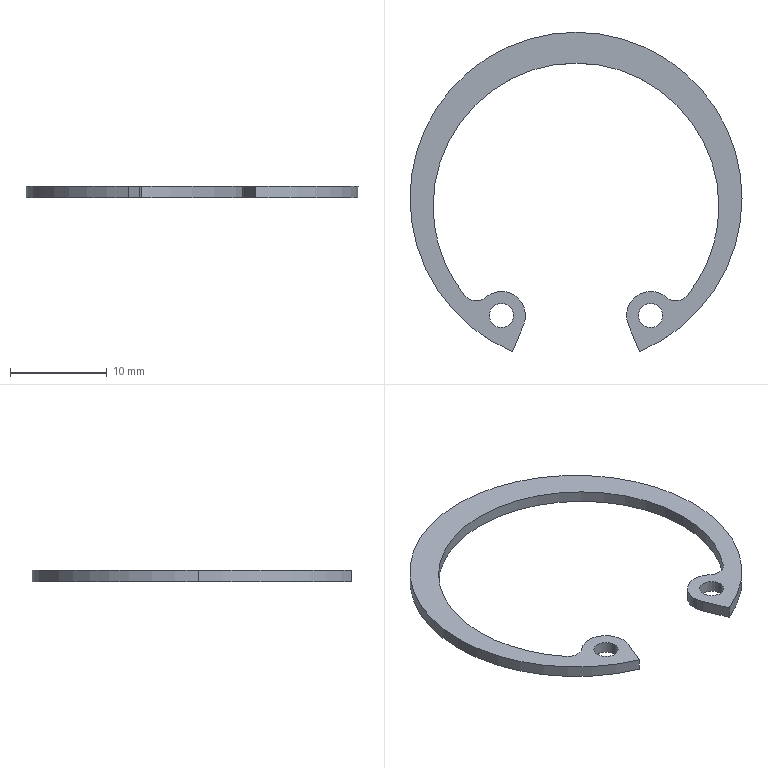Part | SolidWorks | features Extrusion 1 | 1 solid | 19 faces | box 34.4 x 33.091 x 1.2 mm | volume 290.13 mm3 | cylinder 15 | plane 4 | commonest cylinder face diameters 2.5 x4 5 x3 29.6 x3 34.4 x3 3 x2
STEP:
#1=CARTESIAN_POINT('',(6.487,-12.145,-1.2));
#2=VERTEX_POINT('',#1);
#3=CARTESIAN_POINT('',(8.987,-12.145,-1.2));
#4=VERTEX_POINT('',#3);
#5=CARTESIAN_POINT('',(7.737,-12.145,-1.2));
#6=DIRECTION('',(0.,0.,1.));
#7=DIRECTION('',(-1.,0.,0.));
#8=AXIS2_PLACEMENT_3D('',#5,#6,#7);
#9=CIRCLE('',#8,1.25);
#10=EDGE_CURVE('',#2,#4,#9,.T.);
#11=ORIENTED_EDGE('',*,*,#10,.F.);
#12=CARTESIAN_POINT('',(6.487,-12.145,0.));
#13=VERTEX_POINT('',#12);
#14=CARTESIAN_POINT('',(6.487,-12.145,-1.2));
#15=DIRECTION('',(0.,0.,1.));
#16=VECTOR('',#15,1000.);
#17=LINE('',#14,#16);
#18=EDGE_CURVE('',#2,#13,#17,.T.);
#19=ORIENTED_EDGE('',*,*,#18,.T.);
#20=CARTESIAN_POINT('',(8.987,-12.145,0.));
#21=VERTEX_POINT('',#20);
#22=CARTESIAN_POINT('',(7.737,-12.145,0.));
#23=DIRECTION('',(0.,0.,1.));
#24=DIRECTION('',(-1.,0.,0.));
#25=AXIS2_PLACEMENT_3D('',#22,#23,#24);
#26=CIRCLE('',#25,1.25);
#27=EDGE_CURVE('',#13,#21,#26,.T.);
#28=ORIENTED_EDGE('',*,*,#27,.T.);
#29=CARTESIAN_POINT('',(8.987,-12.145,-1.2));
#30=DIRECTION('',(0.,0.,1.));
#31=VECTOR('',#30,1000.);
#32=LINE('',#29,#31);
#33=EDGE_CURVE('',#4,#21,#32,.T.);
#34=ORIENTED_EDGE('',*,*,#33,.F.);
#35=EDGE_LOOP('',(#11,#19,#28,#34));
#36=FACE_OUTER_BOUND('',#35,.T.);
#37=CARTESIAN_POINT('',(7.737,-12.145,-1.2));
#38=DIRECTION('',(0.,0.,1.));
#39=DIRECTION('',(1.,0.,0.));
#40=AXIS2_PLACEMENT_3D('',#37,#38,#39);
#41=CYLINDRICAL_SURFACE('',#40,1.25);
#42=ADVANCED_FACE('',(#36),#41,.F.);
#43=CARTESIAN_POINT('',(-8.987,-12.145,-1.2));
#44=VERTEX_POINT('',#43);
#45=CARTESIAN_POINT('',(-6.487,-12.145,-1.2));
#46=VERTEX_POINT('',#45);
#47=CARTESIAN_POINT('',(-7.737,-12.145,-1.2));
#48=DIRECTION('',(0.,0.,1.));
#49=DIRECTION('',(-1.,0.,0.));
#50=AXIS2_PLACEMENT_3D('',#47,#48,#49);
#51=CIRCLE('',#50,1.25);
#52=EDGE_CURVE('',#44,#46,#51,.T.);
#53=ORIENTED_EDGE('',*,*,#52,.F.);
#54=CARTESIAN_POINT('',(-8.987,-12.145,0.));
#55=VERTEX_POINT('',#54);
#56=CARTESIAN_POINT('',(-8.987,-12.145,-1.2));
#57=DIRECTION('',(0.,0.,1.));
#58=VECTOR('',#57,1000.);
#59=LINE('',#56,#58);
#60=EDGE_CURVE('',#44,#55,#59,.T.);
#61=ORIENTED_EDGE('',*,*,#60,.T.);
#62=CARTESIAN_POINT('',(-6.487,-12.145,0.));
#63=VERTEX_POINT('',#62);
#64=CARTESIAN_POINT('',(-7.737,-12.145,0.));
#65=DIRECTION('',(0.,0.,1.));
#66=DIRECTION('',(-1.,0.,0.));
#67=AXIS2_PLACEMENT_3D('',#64,#65,#66);
#68=CIRCLE('',#67,1.25);
#69=EDGE_CURVE('',#55,#63,#68,.T.);
#70=ORIENTED_EDGE('',*,*,#69,.T.);
#71=CARTESIAN_POINT('',(-6.487,-12.145,-1.2));
#72=DIRECTION('',(0.,0.,1.));
#73=VECTOR('',#72,1000.);
#74=LINE('',#71,#73);
#75=EDGE_CURVE('',#46,#63,#74,.T.);
#76=ORIENTED_EDGE('',*,*,#75,.F.);
#77=EDGE_LOOP('',(#53,#61,#70,#76));
#78=FACE_OUTER_BOUND('',#77,.T.);
#79=CARTESIAN_POINT('',(-7.737,-12.145,-1.2));
#80=DIRECTION('',(0.,0.,1.));
#81=DIRECTION('',(1.,0.,0.));
#82=AXIS2_PLACEMENT_3D('',#79,#80,#81);
#83=CYLINDRICAL_SURFACE('',#82,1.25);
#84=ADVANCED_FACE('',(#78),#83,.F.);
#85=CARTESIAN_POINT('',(17.2,0.,-1.2));
#86=VERTEX_POINT('',#85);
#87=CARTESIAN_POINT('',(-17.2,0.,-1.2));
#88=VERTEX_POINT('',#87);
#89=CARTESIAN_POINT('',(0.,0.,-1.2));
#90=DIRECTION('',(0.,0.,1.));
#91=DIRECTION('',(1.,0.,0.));
#92=AXIS2_PLACEMENT_3D('',#89,#90,#91);
#93=CIRCLE('',#92,17.2);
#94=EDGE_CURVE('',#86,#88,#93,.T.);
#95=ORIENTED_EDGE('',*,*,#94,.T.);
#96=CARTESIAN_POINT('',(-17.2,0.,0.));
#97=VERTEX_POINT('',#96);
#98=CARTESIAN_POINT('',(-17.2,0.,-1.2));
#99=DIRECTION('',(0.,0.,1.));
#100=VECTOR('',#99,1000.);
#101=LINE('',#98,#100);
#102=EDGE_CURVE('',#88,#97,#101,.T.);
#103=ORIENTED_EDGE('',*,*,#102,.T.);
#104=CARTESIAN_POINT('',(17.2,0.,0.));
#105=VERTEX_POINT('',#104);
#106=CARTESIAN_POINT('',(0.,0.,0.));
#107=DIRECTION('',(0.,0.,1.));
#108=DIRECTION('',(1.,0.,0.));
#109=AXIS2_PLACEMENT_3D('',#106,#107,#108);
#110=CIRCLE('',#109,17.2);
#111=EDGE_CURVE('',#105,#97,#110,.T.);
#112=ORIENTED_EDGE('',*,*,#111,.F.);
#113=CARTESIAN_POINT('',(17.2,0.,-1.2));
#114=DIRECTION('',(0.,0.,1.));
#115=VECTOR('',#114,1000.);
#116=LINE('',#113,#115);
#117=EDGE_CURVE('',#86,#105,#116,.T.);
#118=ORIENTED_EDGE('',*,*,#117,.F.);
#119=EDGE_LOOP('',(#95,#103,#112,#118));
#120=FACE_OUTER_BOUND('',#119,.T.);
#121=CARTESIAN_POINT('',(0.,0.,-1.2));
#122=DIRECTION('',(0.,0.,1.));
#123=DIRECTION('',(1.,0.,0.));
#124=AXIS2_PLACEMENT_3D('',#121,#122,#123);
#125=CYLINDRICAL_SURFACE('',#124,17.2);
#126=ADVANCED_FACE('',(#120),#125,.T.);
#127=CARTESIAN_POINT('',(6.582,-15.891,-1.2));
#128=VERTEX_POINT('',#127);
#129=CARTESIAN_POINT('',(0.,0.,-1.2));
#130=DIRECTION('',(0.,0.,1.));
#131=DIRECTION('',(1.,0.,0.));
#132=AXIS2_PLACEMENT_3D('',#129,#130,#131);
#133=CIRCLE('',#132,17.2);
#134=EDGE_CURVE('',#128,#86,#133,.T.);
#135=ORIENTED_EDGE('',*,*,#134,.T.);
#136=ORIENTED_EDGE('',*,*,#117,.T.);
#137=CARTESIAN_POINT('',(6.582,-15.891,0.));
#138=VERTEX_POINT('',#137);
#139=CARTESIAN_POINT('',(0.,0.,0.));
#140=DIRECTION('',(0.,0.,1.));
#141=DIRECTION('',(1.,0.,0.));
#142=AXIS2_PLACEMENT_3D('',#139,#140,#141);
#143=CIRCLE('',#142,17.2);
#144=EDGE_CURVE('',#138,#105,#143,.T.);
#145=ORIENTED_EDGE('',*,*,#144,.F.);
#146=CARTESIAN_POINT('',(6.582,-15.891,-1.2));
#147=DIRECTION('',(0.,0.,1.));
#148=VECTOR('',#147,1000.);
#149=LINE('',#146,#148);
#150=EDGE_CURVE('',#128,#138,#149,.T.);
#151=ORIENTED_EDGE('',*,*,#150,.F.);
#152=EDGE_LOOP('',(#135,#136,#145,#151));
#153=FACE_OUTER_BOUND('',#152,.T.);
#154=CARTESIAN_POINT('',(0.,0.,-1.2));
#155=DIRECTION('',(0.,0.,1.));
#156=DIRECTION('',(1.,0.,0.));
#157=AXIS2_PLACEMENT_3D('',#154,#155,#156);
#158=CYLINDRICAL_SURFACE('',#157,17.2);
#159=ADVANCED_FACE('',(#153),#158,.T.);
#160=CARTESIAN_POINT('',(-5.427,-13.102,-1.2));
#161=VERTEX_POINT('',#160);
#162=CARTESIAN_POINT('',(-5.237,-12.145,-1.2));
#163=VERTEX_POINT('',#162);
#164=CARTESIAN_POINT('',(-7.737,-12.145,-1.2));
#165=DIRECTION('',(0.,0.,1.));
#166=DIRECTION('',(1.,0.,0.));
#167=AXIS2_PLACEMENT_3D('',#164,#165,#166);
#168=CIRCLE('',#167,2.5);
#169=EDGE_CURVE('',#161,#163,#168,.T.);
#170=ORIENTED_EDGE('',*,*,#169,.T.);
#171=CARTESIAN_POINT('',(-5.237,-12.145,0.));
#172=VERTEX_POINT('',#171);
#173=CARTESIAN_POINT('',(-5.237,-12.145,-1.2));
#174=DIRECTION('',(0.,0.,1.));
#175=VECTOR('',#174,1000.);
#176=LINE('',#173,#175);
#177=EDGE_CURVE('',#163,#172,#176,.T.);
#178=ORIENTED_EDGE('',*,*,#177,.T.);
#179=CARTESIAN_POINT('',(-5.427,-13.102,0.));
#180=VERTEX_POINT('',#179);
#181=CARTESIAN_POINT('',(-7.737,-12.145,0.));
#182=DIRECTION('',(0.,0.,1.));
#183=DIRECTION('',(1.,0.,0.));
#184=AXIS2_PLACEMENT_3D('',#181,#182,#183);
#185=CIRCLE('',#184,2.5);
#186=EDGE_CURVE('',#180,#172,#185,.T.);
#187=ORIENTED_EDGE('',*,*,#186,.F.);
#188=CARTESIAN_POINT('',(-5.427,-13.102,-1.2));
#189=DIRECTION('',(0.,0.,1.));
#190=VECTOR('',#189,1000.);
#191=LINE('',#188,#190);
#192=EDGE_CURVE('',#161,#180,#191,.T.);
#193=ORIENTED_EDGE('',*,*,#192,.F.);
#194=EDGE_LOOP('',(#170,#178,#187,#193));
#195=FACE_OUTER_BOUND('',#194,.T.);
#196=CARTESIAN_POINT('',(-7.737,-12.145,-1.2));
#197=DIRECTION('',(0.,0.,1.));
#198=DIRECTION('',(1.,0.,0.));
#199=AXIS2_PLACEMENT_3D('',#196,#197,#198);
#200=CYLINDRICAL_SURFACE('',#199,2.5);
#201=ADVANCED_FACE('',(#195),#200,.T.);
#202=CARTESIAN_POINT('',(-11.536,-10.071,-1.2));
#203=VERTEX_POINT('',#202);
#204=CARTESIAN_POINT('',(-14.8,-0.8,-1.2));
#205=VERTEX_POINT('',#204);
#206=CARTESIAN_POINT('',(0.,-0.8,-1.2));
#207=DIRECTION('',(0.,0.,-1.));
#208=DIRECTION('',(-1.,0.,0.));
#209=AXIS2_PLACEMENT_3D('',#206,#207,#208);
#210=CIRCLE('',#209,14.8);
#211=EDGE_CURVE('',#203,#205,#210,.T.);
#212=ORIENTED_EDGE('',*,*,#211,.T.);
#213=CARTESIAN_POINT('',(-14.8,-0.8,0.));
#214=VERTEX_POINT('',#213);
#215=CARTESIAN_POINT('',(-14.8,-0.8,-1.2));
#216=DIRECTION('',(0.,0.,1.));
#217=VECTOR('',#216,1000.);
#218=LINE('',#215,#217);
#219=EDGE_CURVE('',#205,#214,#218,.T.);
#220=ORIENTED_EDGE('',*,*,#219,.T.);
#221=CARTESIAN_POINT('',(-11.536,-10.071,0.));
#222=VERTEX_POINT('',#221);
#223=CARTESIAN_POINT('',(0.,-0.8,0.));
#224=DIRECTION('',(0.,0.,-1.));
#225=DIRECTION('',(-1.,0.,0.));
#226=AXIS2_PLACEMENT_3D('',#223,#224,#225);
#227=CIRCLE('',#226,14.8);
#228=EDGE_CURVE('',#222,#214,#227,.T.);
#229=ORIENTED_EDGE('',*,*,#228,.F.);
#230=CARTESIAN_POINT('',(-11.536,-10.071,-1.2));
#231=DIRECTION('',(0.,0.,1.));
#232=VECTOR('',#231,1000.);
#233=LINE('',#230,#232);
#234=EDGE_CURVE('',#203,#222,#233,.T.);
#235=ORIENTED_EDGE('',*,*,#234,.F.);
#236=EDGE_LOOP('',(#212,#220,#229,#235));
#237=FACE_OUTER_BOUND('',#236,.T.);
#238=CARTESIAN_POINT('',(0.,-0.8,-1.2));
#239=DIRECTION('',(0.,0.,1.));
#240=DIRECTION('',(1.,0.,0.));
#241=AXIS2_PLACEMENT_3D('',#238,#239,#240);
#242=CYLINDRICAL_SURFACE('',#241,14.8);
#243=ADVANCED_FACE('',(#237),#242,.F.);
#244=ORIENTED_EDGE('',*,*,#219,.F.);
#245=CARTESIAN_POINT('',(14.8,-0.8,-1.2));
#246=VERTEX_POINT('',#245);
#247=CARTESIAN_POINT('',(0.,-0.8,-1.2));
#248=DIRECTION('',(0.,0.,-1.));
#249=DIRECTION('',(-1.,0.,0.));
#250=AXIS2_PLACEMENT_3D('',#247,#248,#249);
#251=CIRCLE('',#250,14.8);
#252=EDGE_CURVE('',#205,#246,#251,.T.);
#253=ORIENTED_EDGE('',*,*,#252,.T.);
#254=CARTESIAN_POINT('',(14.8,-0.8,0.));
#255=VERTEX_POINT('',#254);
#256=CARTESIAN_POINT('',(14.8,-0.8,-1.2));
#257=DIRECTION('',(0.,0.,1.));
#258=VECTOR('',#257,1000.);
#259=LINE('',#256,#258);
#260=EDGE_CURVE('',#246,#255,#259,.T.);
#261=ORIENTED_EDGE('',*,*,#260,.T.);
#262=CARTESIAN_POINT('',(0.,-0.8,0.));
#263=DIRECTION('',(0.,0.,-1.));
#264=DIRECTION('',(-1.,0.,0.));
#265=AXIS2_PLACEMENT_3D('',#262,#263,#264);
#266=CIRCLE('',#265,14.8);
#267=EDGE_CURVE('',#214,#255,#266,.T.);
#268=ORIENTED_EDGE('',*,*,#267,.F.);
#269=EDGE_LOOP('',(#244,#253,#261,#268));
#270=FACE_OUTER_BOUND('',#269,.T.);
#271=CARTESIAN_POINT('',(0.,-0.8,-1.2));
#272=DIRECTION('',(0.,0.,1.));
#273=DIRECTION('',(1.,0.,0.));
#274=AXIS2_PLACEMENT_3D('',#271,#272,#273);
#275=CYLINDRICAL_SURFACE('',#274,14.8);
#276=ADVANCED_FACE('',(#270),#275,.F.);
#277=CARTESIAN_POINT('',(11.536,-10.071,0.));
#278=VERTEX_POINT('',#277);
#279=CARTESIAN_POINT('',(9.381,-10.262,0.));
#280=VERTEX_POINT('',#279);
#281=CARTESIAN_POINT('',(10.367,-9.132,0.));
#282=DIRECTION('',(0.,0.,-1.));
#283=DIRECTION('',(-1.,0.,0.));
#284=AXIS2_PLACEMENT_3D('',#281,#282,#283);
#285=CIRCLE('',#284,1.5);
#286=EDGE_CURVE('',#278,#280,#285,.T.);
#287=ORIENTED_EDGE('',*,*,#286,.F.);
#288=CARTESIAN_POINT('',(11.536,-10.071,-1.2));
#289=VERTEX_POINT('',#288);
#290=CARTESIAN_POINT('',(11.536,-10.071,-1.2));
#291=DIRECTION('',(0.,0.,1.));
#292=VECTOR('',#291,1000.);
#293=LINE('',#290,#292);
#294=EDGE_CURVE('',#289,#278,#293,.T.);
#295=ORIENTED_EDGE('',*,*,#294,.F.);
#296=CARTESIAN_POINT('',(9.381,-10.262,-1.2));
#297=VERTEX_POINT('',#296);
#298=CARTESIAN_POINT('',(10.367,-9.132,-1.2));
#299=DIRECTION('',(0.,0.,-1.));
#300=DIRECTION('',(-1.,0.,0.));
#301=AXIS2_PLACEMENT_3D('',#298,#299,#300);
#302=CIRCLE('',#301,1.5);
#303=EDGE_CURVE('',#289,#297,#302,.T.);
#304=ORIENTED_EDGE('',*,*,#303,.T.);
#305=CARTESIAN_POINT('',(9.381,-10.262,-1.2));
#306=DIRECTION('',(0.,0.,1.));
#307=VECTOR('',#306,1000.);
#308=LINE('',#305,#307);
#309=EDGE_CURVE('',#297,#280,#308,.T.);
#310=ORIENTED_EDGE('',*,*,#309,.T.);
#311=EDGE_LOOP('',(#287,#295,#304,#310));
#312=FACE_OUTER_BOUND('',#311,.T.);
#313=CARTESIAN_POINT('',(10.367,-9.132,-1.2));
#314=DIRECTION('',(0.,0.,1.));
#315=DIRECTION('',(1.,0.,0.));
#316=AXIS2_PLACEMENT_3D('',#313,#314,#315);
#317=CYLINDRICAL_SURFACE('',#316,1.5);
#318=ADVANCED_FACE('',(#312),#317,.F.);
#319=ORIENTED_EDGE('',*,*,#260,.F.);
#320=CARTESIAN_POINT('',(0.,-0.8,-1.2));
#321=DIRECTION('',(0.,0.,-1.));
#322=DIRECTION('',(-1.,0.,0.));
#323=AXIS2_PLACEMENT_3D('',#320,#321,#322);
#324=CIRCLE('',#323,14.8);
#325=EDGE_CURVE('',#246,#289,#324,.T.);
#326=ORIENTED_EDGE('',*,*,#325,.T.);
#327=ORIENTED_EDGE('',*,*,#294,.T.);
#328=CARTESIAN_POINT('',(0.,-0.8,0.));
#329=DIRECTION('',(0.,0.,-1.));
#330=DIRECTION('',(-1.,0.,0.));
#331=AXIS2_PLACEMENT_3D('',#328,#329,#330);
#332=CIRCLE('',#331,14.8);
#333=EDGE_CURVE('',#255,#278,#332,.T.);
#334=ORIENTED_EDGE('',*,*,#333,.F.);
#335=EDGE_LOOP('',(#319,#326,#327,#334));
#336=FACE_OUTER_BOUND('',#335,.T.);
#337=CARTESIAN_POINT('',(0.,-0.8,-1.2));
#338=DIRECTION('',(0.,0.,1.));
#339=DIRECTION('',(1.,0.,0.));
#340=AXIS2_PLACEMENT_3D('',#337,#338,#339);
#341=CYLINDRICAL_SURFACE('',#340,14.8);
#342=ADVANCED_FACE('',(#336),#341,.F.);
#343=CARTESIAN_POINT('',(-9.381,-10.262,0.));
#344=VERTEX_POINT('',#343);
#345=CARTESIAN_POINT('',(-10.367,-9.132,0.));
#346=DIRECTION('',(0.,0.,-1.));
#347=DIRECTION('',(-1.,0.,0.));
#348=AXIS2_PLACEMENT_3D('',#345,#346,#347);
#349=CIRCLE('',#348,1.5);
#350=EDGE_CURVE('',#344,#222,#349,.T.);
#351=ORIENTED_EDGE('',*,*,#350,.F.);
#352=CARTESIAN_POINT('',(-9.381,-10.262,-1.2));
#353=VERTEX_POINT('',#352);
#354=CARTESIAN_POINT('',(-9.381,-10.262,-1.2));
#355=DIRECTION('',(0.,0.,1.));
#356=VECTOR('',#355,1000.);
#357=LINE('',#354,#356);
#358=EDGE_CURVE('',#353,#344,#357,.T.);
#359=ORIENTED_EDGE('',*,*,#358,.F.);
#360=CARTESIAN_POINT('',(-10.367,-9.132,-1.2));
#361=DIRECTION('',(0.,0.,-1.));
#362=DIRECTION('',(-1.,0.,0.));
#363=AXIS2_PLACEMENT_3D('',#360,#361,#362);
#364=CIRCLE('',#363,1.5);
#365=EDGE_CURVE('',#353,#203,#364,.T.);
#366=ORIENTED_EDGE('',*,*,#365,.T.);
#367=ORIENTED_EDGE('',*,*,#234,.T.);
#368=EDGE_LOOP('',(#351,#359,#366,#367));
#369=FACE_OUTER_BOUND('',#368,.T.);
#370=CARTESIAN_POINT('',(-10.367,-9.132,-1.2));
#371=DIRECTION('',(0.,0.,1.));
#372=DIRECTION('',(1.,0.,0.));
#373=AXIS2_PLACEMENT_3D('',#370,#371,#372);
#374=CYLINDRICAL_SURFACE('',#373,1.5);
#375=ADVANCED_FACE('',(#369),#374,.F.);
#376=ORIENTED_EDGE('',*,*,#177,.F.);
#377=CARTESIAN_POINT('',(-7.737,-12.145,-1.2));
#378=DIRECTION('',(0.,0.,1.));
#379=DIRECTION('',(1.,0.,0.));
#380=AXIS2_PLACEMENT_3D('',#377,#378,#379);
#381=CIRCLE('',#380,2.5);
#382=EDGE_CURVE('',#163,#353,#381,.T.);
#383=ORIENTED_EDGE('',*,*,#382,.T.);
#384=ORIENTED_EDGE('',*,*,#358,.T.);
#385=CARTESIAN_POINT('',(-7.737,-12.145,0.));
#386=DIRECTION('',(0.,0.,1.));
#387=DIRECTION('',(1.,0.,0.));
#388=AXIS2_PLACEMENT_3D('',#385,#386,#387);
#389=CIRCLE('',#388,2.5);
#390=EDGE_CURVE('',#172,#344,#389,.T.);
#391=ORIENTED_EDGE('',*,*,#390,.F.);
#392=EDGE_LOOP('',(#376,#383,#384,#391));
#393=FACE_OUTER_BOUND('',#392,.T.);
#394=CARTESIAN_POINT('',(-7.737,-12.145,-1.2));
#395=DIRECTION('',(0.,0.,1.));
#396=DIRECTION('',(1.,0.,0.));
#397=AXIS2_PLACEMENT_3D('',#394,#395,#396);
#398=CYLINDRICAL_SURFACE('',#397,2.5);
#399=ADVANCED_FACE('',(#393),#398,.T.);
#400=CARTESIAN_POINT('',(-6.582,-15.891,0.));
#401=VERTEX_POINT('',#400);
#402=CARTESIAN_POINT('',(-6.582,-15.891,0.));
#403=DIRECTION('',(0.3827,0.9239,0.));
#404=VECTOR('',#403,1000.);
#405=LINE('',#402,#404);
#406=EDGE_CURVE('',#401,#180,#405,.T.);
#407=ORIENTED_EDGE('',*,*,#406,.F.);
#408=CARTESIAN_POINT('',(-6.582,-15.891,-1.2));
#409=VERTEX_POINT('',#408);
#410=CARTESIAN_POINT('',(-6.582,-15.891,-1.2));
#411=DIRECTION('',(0.,0.,1.));
#412=VECTOR('',#411,1000.);
#413=LINE('',#410,#412);
#414=EDGE_CURVE('',#409,#401,#413,.T.);
#415=ORIENTED_EDGE('',*,*,#414,.F.);
#416=CARTESIAN_POINT('',(-6.582,-15.891,-1.2));
#417=DIRECTION('',(0.3827,0.9239,0.));
#418=VECTOR('',#417,1000.);
#419=LINE('',#416,#418);
#420=EDGE_CURVE('',#409,#161,#419,.T.);
#421=ORIENTED_EDGE('',*,*,#420,.T.);
#422=ORIENTED_EDGE('',*,*,#192,.T.);
#423=EDGE_LOOP('',(#407,#415,#421,#422));
#424=FACE_OUTER_BOUND('',#423,.T.);
#425=CARTESIAN_POINT('',(-6.582,-15.891,-1.2));
#426=DIRECTION('',(0.9239,-0.3827,0.));
#427=DIRECTION('',(0.3827,0.9239,0.));
#428=AXIS2_PLACEMENT_3D('',#425,#426,#427);
#429=PLANE('',#428);
#430=ADVANCED_FACE('',(#424),#429,.T.);
#431=ORIENTED_EDGE('',*,*,#102,.F.);
#432=CARTESIAN_POINT('',(0.,0.,-1.2));
#433=DIRECTION('',(0.,0.,1.));
#434=DIRECTION('',(1.,0.,0.));
#435=AXIS2_PLACEMENT_3D('',#432,#433,#434);
#436=CIRCLE('',#435,17.2);
#437=EDGE_CURVE('',#88,#409,#436,.T.);
#438=ORIENTED_EDGE('',*,*,#437,.T.);
#439=ORIENTED_EDGE('',*,*,#414,.T.);
#440=CARTESIAN_POINT('',(0.,0.,0.));
#441=DIRECTION('',(0.,0.,1.));
#442=DIRECTION('',(1.,0.,0.));
#443=AXIS2_PLACEMENT_3D('',#440,#441,#442);
#444=CIRCLE('',#443,17.2);
#445=EDGE_CURVE('',#97,#401,#444,.T.);
#446=ORIENTED_EDGE('',*,*,#445,.F.);
#447=EDGE_LOOP('',(#431,#438,#439,#446));
#448=FACE_OUTER_BOUND('',#447,.T.);
#449=CARTESIAN_POINT('',(0.,0.,-1.2));
#450=DIRECTION('',(0.,0.,1.));
#451=DIRECTION('',(1.,0.,0.));
#452=AXIS2_PLACEMENT_3D('',#449,#450,#451);
#453=CYLINDRICAL_SURFACE('',#452,17.2);
#454=ADVANCED_FACE('',(#448),#453,.T.);
#455=CARTESIAN_POINT('',(5.427,-13.102,0.));
#456=VERTEX_POINT('',#455);
#457=CARTESIAN_POINT('',(5.427,-13.102,0.));
#458=DIRECTION('',(0.3827,-0.9239,0.));
#459=VECTOR('',#458,1000.);
#460=LINE('',#457,#459);
#461=EDGE_CURVE('',#456,#138,#460,.T.);
#462=ORIENTED_EDGE('',*,*,#461,.F.);
#463=CARTESIAN_POINT('',(5.427,-13.102,-1.2));
#464=VERTEX_POINT('',#463);
#465=CARTESIAN_POINT('',(5.427,-13.102,-1.2));
#466=DIRECTION('',(0.,0.,1.));
#467=VECTOR('',#466,1000.);
#468=LINE('',#465,#467);
#469=EDGE_CURVE('',#464,#456,#468,.T.);
#470=ORIENTED_EDGE('',*,*,#469,.F.);
#471=CARTESIAN_POINT('',(5.427,-13.102,-1.2));
#472=DIRECTION('',(0.3827,-0.9239,0.));
#473=VECTOR('',#472,1000.);
#474=LINE('',#471,#473);
#475=EDGE_CURVE('',#464,#128,#474,.T.);
#476=ORIENTED_EDGE('',*,*,#475,.T.);
#477=ORIENTED_EDGE('',*,*,#150,.T.);
#478=EDGE_LOOP('',(#462,#470,#476,#477));
#479=FACE_OUTER_BOUND('',#478,.T.);
#480=CARTESIAN_POINT('',(5.427,-13.102,-1.2));
#481=DIRECTION('',(-0.9239,-0.3827,0.));
#482=DIRECTION('',(0.3827,-0.9239,0.));
#483=AXIS2_PLACEMENT_3D('',#480,#481,#482);
#484=PLANE('',#483);
#485=ADVANCED_FACE('',(#479),#484,.T.);
#486=CARTESIAN_POINT('',(7.737,-12.145,0.));
#487=DIRECTION('',(0.,0.,1.));
#488=DIRECTION('',(1.,0.,0.));
#489=AXIS2_PLACEMENT_3D('',#486,#487,#488);
#490=CIRCLE('',#489,2.5);
#491=EDGE_CURVE('',#280,#456,#490,.T.);
#492=ORIENTED_EDGE('',*,*,#491,.F.);
#493=ORIENTED_EDGE('',*,*,#309,.F.);
#494=CARTESIAN_POINT('',(7.737,-12.145,-1.2));
#495=DIRECTION('',(0.,0.,1.));
#496=DIRECTION('',(1.,0.,0.));
#497=AXIS2_PLACEMENT_3D('',#494,#495,#496);
#498=CIRCLE('',#497,2.5);
#499=EDGE_CURVE('',#297,#464,#498,.T.);
#500=ORIENTED_EDGE('',*,*,#499,.T.);
#501=ORIENTED_EDGE('',*,*,#469,.T.);
#502=EDGE_LOOP('',(#492,#493,#500,#501));
#503=FACE_OUTER_BOUND('',#502,.T.);
#504=CARTESIAN_POINT('',(7.737,-12.145,-1.2));
#505=DIRECTION('',(0.,0.,1.));
#506=DIRECTION('',(1.,0.,0.));
#507=AXIS2_PLACEMENT_3D('',#504,#505,#506);
#508=CYLINDRICAL_SURFACE('',#507,2.5);
#509=ADVANCED_FACE('',(#503),#508,.T.);
#510=CARTESIAN_POINT('',(7.737,-12.145,-1.2));
#511=DIRECTION('',(0.,0.,1.));
#512=DIRECTION('',(-1.,0.,0.));
#513=AXIS2_PLACEMENT_3D('',#510,#511,#512);
#514=CIRCLE('',#513,1.25);
#515=EDGE_CURVE('',#4,#2,#514,.T.);
#516=ORIENTED_EDGE('',*,*,#515,.T.);
#517=ORIENTED_EDGE('',*,*,#10,.T.);
#518=EDGE_LOOP('',(#516,#517));
#519=FACE_BOUND('',#518,.T.);
#520=CARTESIAN_POINT('',(-7.737,-12.145,-1.2));
#521=DIRECTION('',(0.,0.,1.));
#522=DIRECTION('',(-1.,0.,0.));
#523=AXIS2_PLACEMENT_3D('',#520,#521,#522);
#524=CIRCLE('',#523,1.25);
#525=EDGE_CURVE('',#46,#44,#524,.T.);
#526=ORIENTED_EDGE('',*,*,#525,.T.);
#527=ORIENTED_EDGE('',*,*,#52,.T.);
#528=EDGE_LOOP('',(#526,#527));
#529=FACE_BOUND('',#528,.T.);
#530=ORIENTED_EDGE('',*,*,#303,.F.);
#531=ORIENTED_EDGE('',*,*,#325,.F.);
#532=ORIENTED_EDGE('',*,*,#252,.F.);
#533=ORIENTED_EDGE('',*,*,#211,.F.);
#534=ORIENTED_EDGE('',*,*,#365,.F.);
#535=ORIENTED_EDGE('',*,*,#382,.F.);
#536=ORIENTED_EDGE('',*,*,#169,.F.);
#537=ORIENTED_EDGE('',*,*,#420,.F.);
#538=ORIENTED_EDGE('',*,*,#437,.F.);
#539=ORIENTED_EDGE('',*,*,#94,.F.);
#540=ORIENTED_EDGE('',*,*,#134,.F.);
#541=ORIENTED_EDGE('',*,*,#475,.F.);
#542=ORIENTED_EDGE('',*,*,#499,.F.);
#543=EDGE_LOOP('',(#530,#531,#532,#533,#534,#535,#536,#537,#538,#539,#540,#541,#542));
#544=FACE_OUTER_BOUND('',#543,.T.);
#545=CARTESIAN_POINT('',(10.367,-9.132,-1.2));
#546=DIRECTION('',(0.,0.,-1.));
#547=DIRECTION('',(-1.,0.,0.));
#548=AXIS2_PLACEMENT_3D('',#545,#546,#547);
#549=PLANE('',#548);
#550=ADVANCED_FACE('',(#519,#529,#544),#549,.T.);
#551=CARTESIAN_POINT('',(7.737,-12.145,0.));
#552=DIRECTION('',(0.,0.,1.));
#553=DIRECTION('',(-1.,0.,0.));
#554=AXIS2_PLACEMENT_3D('',#551,#552,#553);
#555=CIRCLE('',#554,1.25);
#556=EDGE_CURVE('',#21,#13,#555,.T.);
#557=ORIENTED_EDGE('',*,*,#556,.F.);
#558=ORIENTED_EDGE('',*,*,#27,.F.);
#559=EDGE_LOOP('',(#557,#558));
#560=FACE_BOUND('',#559,.T.);
#561=CARTESIAN_POINT('',(-7.737,-12.145,0.));
#562=DIRECTION('',(0.,0.,1.));
#563=DIRECTION('',(-1.,0.,0.));
#564=AXIS2_PLACEMENT_3D('',#561,#562,#563);
#565=CIRCLE('',#564,1.25);
#566=EDGE_CURVE('',#63,#55,#565,.T.);
#567=ORIENTED_EDGE('',*,*,#566,.F.);
#568=ORIENTED_EDGE('',*,*,#69,.F.);
#569=EDGE_LOOP('',(#567,#568));
#570=FACE_BOUND('',#569,.T.);
#571=ORIENTED_EDGE('',*,*,#286,.T.);
#572=ORIENTED_EDGE('',*,*,#491,.T.);
#573=ORIENTED_EDGE('',*,*,#461,.T.);
#574=ORIENTED_EDGE('',*,*,#144,.T.);
#575=ORIENTED_EDGE('',*,*,#111,.T.);
#576=ORIENTED_EDGE('',*,*,#445,.T.);
#577=ORIENTED_EDGE('',*,*,#406,.T.);
#578=ORIENTED_EDGE('',*,*,#186,.T.);
#579=ORIENTED_EDGE('',*,*,#390,.T.);
#580=ORIENTED_EDGE('',*,*,#350,.T.);
#581=ORIENTED_EDGE('',*,*,#228,.T.);
#582=ORIENTED_EDGE('',*,*,#267,.T.);
#583=ORIENTED_EDGE('',*,*,#333,.T.);
#584=EDGE_LOOP('',(#571,#572,#573,#574,#575,#576,#577,#578,#579,#580,#581,#582,#583));
#585=FACE_OUTER_BOUND('',#584,.T.);
#586=CARTESIAN_POINT('',(10.367,-9.132,0.));
#587=DIRECTION('',(0.,0.,-1.));
#588=DIRECTION('',(-1.,0.,0.));
#589=AXIS2_PLACEMENT_3D('',#586,#587,#588);
#590=PLANE('',#589);
#591=ADVANCED_FACE('',(#560,#570,#585),#590,.F.);
#592=ORIENTED_EDGE('',*,*,#60,.F.);
#593=ORIENTED_EDGE('',*,*,#525,.F.);
#594=ORIENTED_EDGE('',*,*,#75,.T.);
#595=ORIENTED_EDGE('',*,*,#566,.T.);
#596=EDGE_LOOP('',(#592,#593,#594,#595));
#597=FACE_OUTER_BOUND('',#596,.T.);
#598=CARTESIAN_POINT('',(-7.737,-12.145,-1.2));
#599=DIRECTION('',(0.,0.,1.));
#600=DIRECTION('',(1.,0.,0.));
#601=AXIS2_PLACEMENT_3D('',#598,#599,#600);
#602=CYLINDRICAL_SURFACE('',#601,1.25);
#603=ADVANCED_FACE('',(#597),#602,.F.);
#604=ORIENTED_EDGE('',*,*,#18,.F.);
#605=ORIENTED_EDGE('',*,*,#515,.F.);
#606=ORIENTED_EDGE('',*,*,#33,.T.);
#607=ORIENTED_EDGE('',*,*,#556,.T.);
#608=EDGE_LOOP('',(#604,#605,#606,#607));
#609=FACE_OUTER_BOUND('',#608,.T.);
#610=CARTESIAN_POINT('',(7.737,-12.145,-1.2));
#611=DIRECTION('',(0.,0.,1.));
#612=DIRECTION('',(1.,0.,0.));
#613=AXIS2_PLACEMENT_3D('',#610,#611,#612);
#614=CYLINDRICAL_SURFACE('',#613,1.25);
#615=ADVANCED_FACE('',(#609),#614,.F.);
#616=CLOSED_SHELL('',(#42,#84,#126,#159,#201,#243,#276,#318,#342,#375,#399,#430,#454,#485,#509,#550,#591,#603,#615));
#617=MANIFOLD_SOLID_BREP('',#616);
#618=CARTESIAN_POINT('',(0.,0.,0.));
#619=DIRECTION('',(0.,0.,1.));
#620=DIRECTION('',(1.,0.,0.));
#621=AXIS2_PLACEMENT_3D('',#618,#619,#620);
#622=(LENGTH_UNIT()NAMED_UNIT(*)SI_UNIT(.MILLI.,.METRE.));
#623=UNCERTAINTY_MEASURE_WITH_UNIT(LENGTH_MEASURE(0.00001),#622,'','');
#624=(NAMED_UNIT(*)PLANE_ANGLE_UNIT()SI_UNIT($,.RADIAN.));
#625=(NAMED_UNIT(*)SI_UNIT($,.STERADIAN.)SOLID_ANGLE_UNIT());
#626=(GEOMETRIC_REPRESENTATION_CONTEXT(3)GLOBAL_UNCERTAINTY_ASSIGNED_CONTEXT((#623))GLOBAL_UNIT_ASSIGNED_CONTEXT((#622,#624,#625))REPRESENTATION_CONTEXT('',''));
#627=ADVANCED_BREP_SHAPE_REPRESENTATION('',(#617,#621),#626);